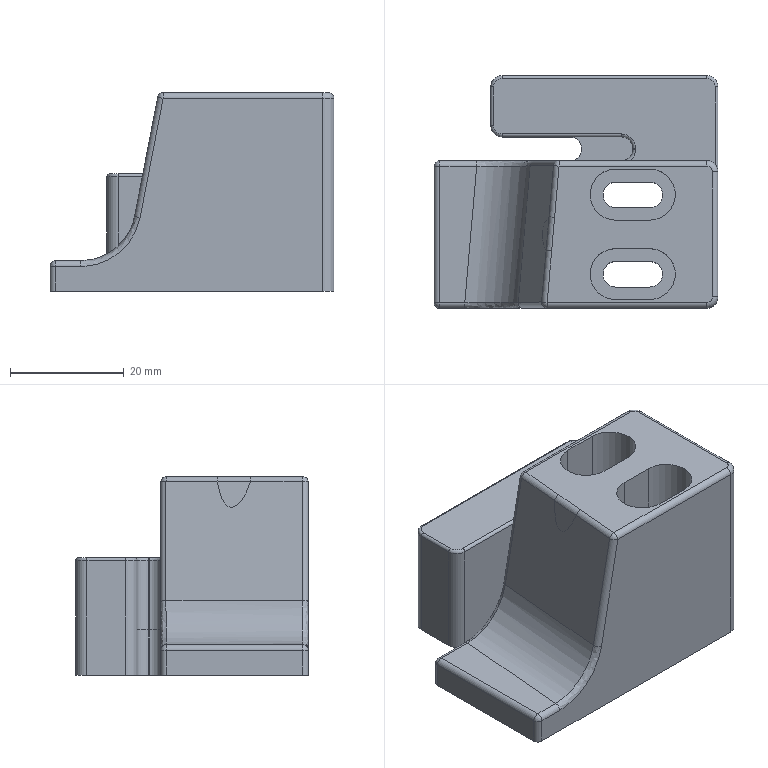NC program | NX | posted with a generic post | part box 50 x 41 x 35 mm
Lines 5590 to 6591 of 6591:
(CAVITY_MILL_COPY_COPY , TOOL : D4)
N11154 T04 M6
N11156 G17 G43 G0 G90 X-9.331 Y5.48 Z30. S9500 H4 M3
N11158 Z-14.738
N11160 G94 G1 X-9.129 Y5.481 F1000.
N11162 G3 X-8.265 Y5.984 R1.
N11164 G2 X-5.643 Y7.5 R3.011 F1400.
N11166 G1 X8.004
N11168 Y7.7
N11170 X8. Y7.704
N11172 X-9.144
N11174 G3 X-10.01 Y7.204 R1.
N11176 G1 X-10.184 Y6.904
N11178 G0 X-9.42 Y5.455 Z-15.177
N11180 G1 X-9.217 Y5.456 F1000.
N11182 G3 X-8.355 Y5.963 R1.
N11184 G2 X-5.728 Y7.5 R3.029 F1400.
N11186 G1 X8.
N11188 Y7.7
N11190 X-9.232
N11192 G3 X-10.098 Y7.2 R1.
N11194 G1 X-10.271 Y6.9
N11196 G0 X-9.505 Y5.452 Z-15.615
N11198 G1 X-9.303 Y5.454 F1000.
N11200 G3 X-8.441 Y5.962 R1.
N11202 G2 X-5.812 Y7.5 R3.03 F1400.
N11204 G1 X8.
N11206 Y7.7
N11208 X-9.317
N11210 G3 X-10.183 Y7.2 R1.
N11212 G1 X-10.356 Y6.9
N11214 G0 X-9.589 Y5.455 Z-16.054
N11216 G1 X-9.387 Y5.457 F1000.
N11218 G3 X-8.525 Y5.964 R1.
N11220 G2 X-5.863 Y7.5 R3.03 F1400.
N11222 G1 X8.
N11224 Y7.7
N11226 X-9.401
N11228 G3 X-10.267 Y7.2 R1.
N11230 G1 X-10.44 Y6.9
N11232 G0 X-9.671 Y5.476 Z-16.492
N11234 G1 X-9.469 Y5.477 F1000.
N11236 G3 X-8.606 Y5.981 R1.
N11238 G2 X-5.982 Y7.5 R3.011 F1400.
N11240 G1 X8.
N11242 Y7.7
N11244 X-9.486
N11246 G3 X-10.352 Y7.2 R1.
N11248 G1 X-10.525 Y6.9
N11250 G0 X-9.756 Y5.476 Z-16.931
N11252 G1 X-9.554 Y5.477 F1000.
N11254 G3 X-8.69 Y5.981 R1.
N11256 G2 X-6.067 Y7.5 R3.011 F1400.
N11258 G1 X8.
N11260 Y7.7
N11262 X-9.571
N11264 G3 X-10.437 Y7.2 R1.
N11266 G1 X-10.61 Y6.9
N11268 G0 X-9.843 Y5.457 Z-17.369
N11270 G1 X-9.641 Y5.459 F1000.
N11272 G3 X-8.778 Y5.966 R1.
N11274 G2 X-6.152 Y7.5 R3.028 F1400.
N11276 G1 X8.
N11278 Y7.7
N11280 X-9.655
N11282 G3 X-10.521 Y7.2 R1.
N11284 G1 X-10.695 Y6.9
N11286 G0 X-9.929 Y5.455 Z-17.808
N11288 G1 X-9.726 Y5.456 F1000.
N11290 G3 X-8.864 Y5.964 R1.
N11292 G2 X-6.202 Y7.5 R3.03 F1400.
N11294 G1 X8.
N11296 Y7.7
N11298 X-9.74
N11300 G3 X-10.606 Y7.2 R1.
N11302 G1 X-10.779 Y6.9
N11304 G0 X-10.013 Y5.455 Z-18.246
N11306 G1 X-9.81 Y5.456 F1000.
N11308 G3 X-8.948 Y5.964 R1.
N11310 G2 X-6.321 Y7.5 R3.03 F1400.
N11312 G1 X8.
N11314 Y7.7
N11316 X-9.825
N11318 G3 X-10.691 Y7.2 R1.
N11320 G1 X-10.864 Y6.9
N11322 G0 X-10.095 Y5.475 Z-18.685
N11324 G1 X-9.893 Y5.476 F1000.
N11326 G3 X-9.03 Y5.981 R1.
N11328 G2 X-6.406 Y7.5 R3.011 F1400.
N11330 G1 X8.
N11332 Y7.7
N11334 X-9.91
N11336 G3 X-10.776 Y7.2 R1.
N11338 G1 X-10.949 Y6.9
N11340 G0 X-10.184 Y5.449 Z-19.123
N11342 G1 X-9.98 Y5.451 F1000.
N11344 G3 X-9.119 Y5.959 R1.
N11346 G2 X-6.447 Y7.5 R3.035 F1400.
N11348 G1 X8.
N11350 Y7.7
N11352 X-9.994
N11354 G3 X-10.86 Y7.2 R1.
N11356 G1 X-11.034 Y6.9
N11358 G0 X-10.265 Y5.475 Z-19.562
N11360 G1 X-10.062 Y5.476 F1000.
N11362 G3 X-9.199 Y5.981 R1.
N11364 G2 X-6.575 Y7.5 R3.011 F1400.
N11366 G1 X8.
N11368 Y7.7
N11370 X-10.079
N11372 G3 X-10.945 Y7.2 R1.
N11374 G1 X-11.118 Y6.9
N11376 G0 X-10.351 Y5.455 Z-20.
N11378 G1 X-10.148 Y5.457 F1000.
N11380 G3 X-9.286 Y5.964 R1.
N11382 G2 X-6.659 Y7.5 R3.03 F1400.
N11384 G1 X8.
N11386 Y7.7
N11388 X-10.162
N11390 G3 X-11.029 Y7.2 R1.
N11392 G1 X-11.202 Y6.9
N11394 G0 X-10.437 Y5.453 Z-20.438
N11396 G1 X-10.234 Y5.455 F1000.
N11398 G3 X-9.372 Y5.962 R1.
N11400 G2 X-6.745 Y7.5 R3.031 F1400.
N11402 G1 X8.
N11404 Y7.7
N11406 X-10.248
N11408 G3 X-11.115 Y7.2 R1.
N11410 G1 X-11.288 Y6.9
N11412 G0 X-10.522 Y5.451 Z-20.875
N11414 G1 X-10.319 Y5.453 F1000.
N11416 G3 X-9.458 Y5.961 R1.
N11418 G2 X-6.794 Y7.5 R3.03 F1400.
N11420 G1 X8.
N11422 Y7.7
N11424 X-10.334
N11426 G3 X-11.2 Y7.2 R1.
N11428 G1 X-11.373 Y6.9
N11430 G0 X-10.606 Y5.465 Z-21.313
N11432 G1 X-10.404 Y5.466 F1000.
N11434 G3 X-9.542 Y5.973 R1.
N11436 G2 X-6.914 Y7.5 R3.011 F1400.
N11438 G1 X8.
N11440 Y7.7
N11442 X-10.421
N11444 G3 X-11.287 Y7.2 R1.
N11446 G1 X-11.46 Y6.9
N11448 G0 X-10.696 Y5.431 Z-21.75
N11450 G1 X-10.493 Y5.434 F1000.
N11452 G3 X-9.634 Y5.946 R1.
N11454 G2 X-6.998 Y7.5 R3.034 F1400.
N11456 G1 X8.
N11458 Y7.7
N11460 X-10.508
N11462 G3 X-11.374 Y7.2 R1.
N11464 G1 X-11.547 Y6.9
N11466 G0 X-10.788 Y5.443 Z-22.188
N11468 G1 X-10.586 Y5.446 F1000.
N11470 G3 X-9.727 Y5.958 R1.
N11472 G2 X-7.087 Y7.5 R3.013 F1400.
N11474 G1 X8.
N11476 Y7.7
N11478 X-10.604
N11480 G3 X-11.47 Y7.2 R1.
N11482 G1 X-11.643 Y6.9
N11484 G0 X-10.906 Y5.447 Z-22.625
N11486 G1 X-10.706 Y5.449 F1000.
N11488 G3 X-9.848 Y5.962 R1.
N11490 G2 X-8.516 Y7.198 R2.942 F1400.
N11492 G1 X-8.217 Y7.32
N11494 G2 X-7.189 Y7.5 R3.049
N11496 G1 X8.
N11498 Y7.7
N11500 X-10.726
N11502 G3 X-11.592 Y7.2 R1.
N11504 G1 X-11.765 Y6.9
N11506 G0 X-11.032 Y5.473 Z-23.063
N11508 G1 X-10.831 Y5.474 F1000.
N11510 G3 X-9.968 Y5.979 R1.
N11512 G2 X-8.017 Y7.418 R2.987 F1400.
N11514 X-7.311 Y7.5 R3.335
N11516 G1 X8.
N11518 Y7.7
N11520 X-10.847
N11522 G3 X-11.713 Y7.2 R1.
N11524 G1 X-11.887 Y6.9
N11526 G0 X-11.196 Y5.452 Z-23.5
N11528 G1 X-10.995 Y5.454 F1000.
N11530 G3 X-10.133 Y5.961 R1.
N11532 G2 X-8.477 Y7.32 R2.974 F1400.
N11534 X-7.454 Y7.5 R2.915
N11536 G1 X8.
N11538 Y7.7
N11540 X-11.008
N11542 G3 X-11.874 Y7.2 R1.
N11544 G1 X-12.047 Y6.9
N11546 G0 X-11.4 Y5.448 Z-23.938
N11548 G1 X-11.173 Y5.449 F1000.
N11550 G3 X-10.309 Y5.953 R1.
N11552 G2 X-7.618 Y7.5 R3.072 F1400.
N11554 G1 X8.
N11556 Y7.7
N11558 X-11.181
N11560 G3 X-12.047 Y7.2 R1.
N11562 G1 X-12.22 Y6.9
N11564 G0 X-11.591 Y5.532 Z-24.375
N11566 G1 X-11.431 Y5.519 F1000.
N11568 G3 X-10.527 Y5.947 R1.
N11570 G1 X-10.462 Y6.035 F1400.
N11572 G2 X-9.002 Y7.261 R2.886
N11574 G1 X-8.855 Y7.32
N11576 G2 X-7.805 Y7.5 R3.174
N11578 G1 X8.
N11580 Y7.7
N11582 X-11.392
N11584 G3 X-12.258 Y7.2 R1.
N11586 G1 X-12.431 Y6.9
N11588 G0 X-11.818 Y5.505 Z-24.813
N11590 G1 X-11.622 Y5.502 F1000.
N11592 G3 X-10.748 Y5.989 R1.
N11594 G2 X-9.805 Y6.948 R2.853 F1400.
N11596 G1 X-9.678 Y7.027
N11598 G2 X-8.02 Y7.5 R3.142
N11600 G1 X8.
N11602 Y7.7
N11604 X-11.618
N11606 G3 X-12.484 Y7.2 R1.
N11608 G1 X-12.657 Y6.9
N11610 G0 X-12.106 Y5.475 Z-25.25
N11612 G1 X-11.924 Y5.469 F1000.
N11614 G3 X-11.043 Y5.942 R1.
N11616 G1 X-10.949 Y6.084 F1400.
N11618 G2 X-8.254 Y7.5 R3.263
N11620 G1 X8.
N11622 Y7.7
N11624 X-11.896
N11626 G3 X-12.762 Y7.2 R1.
N11628 G1 X-12.935 Y6.9
N11630 G0 X-12.399 Y5.469 Z-25.688
N11632 G1 X-12.2 Y5.468 F1000.
N11634 G3 X-11.331 Y5.962 R1.
N11636 G2 X-10.441 Y6.907 R2.907 F1400.
N11638 X-8.518 Y7.5 R3.501
N11640 G1 X8.
N11642 Y7.7
N11644 X-12.198
N11646 G3 X-13.064 Y7.2 R1.
N11648 G1 X-13.234 Y6.906
N11650 G0 X-12.742 Y5.449 Z-26.125
N11652 G1 X-12.543 Y5.448 F1000.
N11654 G3 X-11.673 Y5.941 R1.
N11656 G2 X-10.343 Y7.131 R2.923 F1400.
N11658 G1 X-10.116 Y7.232
N11660 G2 X-8.855 Y7.5 R3.099
N11662 G1 X8.
N11664 Y7.7
N11666 X-12.532
N11668 G3 X-13.398 Y7.2 R1.
N11670 G1 X-13.553 Y6.932
N11672 G0 X-13.117 Y5.51 Z-26.563
N11674 G1 X-12.923 Y5.503 F1000.
N11676 G3 X-12.041 Y5.976 R1.
N11678 G2 X-11.64 Y6.48 R2.775 F1400.
N11680 X-9.168 Y7.5 R3.507
N11682 G1 X8.
N11684 Y7.7
N11686 X-12.898
N11688 G3 X-13.764 Y7.2 R1.
N11690 G1 X-13.889 Y6.983
N11692 G0 X-13.612 Y5.249 Z-27.
N11694 G1 X-13.423 Y5.255 F1000.
N11696 G3 X-12.574 Y5.784 R1.
N11698 G2 X-11.99 Y6.523 R2.671 F1400.
N11700 G1 X-11.922 Y6.584
N11702 G2 X-9.501 Y7.5 R3.521
N11704 G1 X8.
N11706 Y7.7
N11708 X-13.
N11710 G2 X-13.364 Y7.717 R4.
N11712 G3 X-14.272 Y7.297 R1.
N11714 G1 X-14.404 Y7.11
N11716 G0 X-14.044 Y5.519 Z-27.433
N11718 G1 X-13.85 Y5.511 F1000.
N11720 G3 X-12.964 Y5.974 R1.
N11722 G2 X-12.264 Y6.721 R2.766 F1400.
N11724 X-9.914 Y7.5 R4.031
N11726 G1 X-1.
N11728 Y7.614
N11730 Y7.7
N11732 X-13.
N11734 G2 X-13.704 Y7.762 R4.
N11736 G3 X-14.645 Y7.423 R1.
N11738 G1 X-14.793 Y7.247
N11740 G0 X-14.588 Y5.601 Z-27.867
N11742 G1 X-14.402 Y5.583 F1000.
N11744 G3 X-13.494 Y6.001 R1.
N11746 G2 X-13.249 Y6.298 R2.59 F1400.
N11748 X-10.335 Y7.5 R3.909
N11750 G1 X-1.
N11752 Y7.614
N11754 Y7.7
N11756 X-13.
N11758 G2 X-14.082 Y7.849 R4.
N11760 G3 X-15.051 Y7.602 R1.
N11762 G1 X-15.216 Y7.442
N11764 G0 X-15.192 Y5.797 Z-28.3
N11766 G1 X-15.008 Y5.768 F1000.
N11768 G3 X-14.074 Y6.126 R1.
N11770 G2 X-13.701 Y6.5 R2.589 F1400.
N11772 X-10.881 Y7.5 R4.428
N11774 G1 X-1.
N11776 Y7.614
N11778 Y7.7
N11780 X-13.
N11782 G2 X-14.5 Y7.992 R4.
N11784 G3 X-15.49 Y7.853 R1.
N11786 G1 X-15.671 Y7.712
N11788 G0 X-15.882 Y6.108 Z-28.733
N11790 G1 X-15.71 Y6.057 F1000.
N11792 G3 X-14.738 Y6.293 R1.
N11794 G1 X-14.686 Y6.34 F1400.
N11796 G2 X-11.471 Y7.5 R4.895
N11798 G1 X-1.
N11800 Y7.614
N11802 Y7.7
N11804 X-13.
N11806 G2 X-14.934 Y8.199 R4.
N11808 G3 X-15.934 Y8.18 R1.
N11810 G1 X-16.13 Y8.061
N11812 G0 X-16.711 Y6.539 Z-29.167
N11814 G1 X-16.521 Y6.444 F1000.
N11816 G3 X-15.523 Y6.505 R1.
N11818 G2 X-12.156 Y7.5 R5.991 F1400.
N11820 G1 X-1.
N11822 Y7.614
N11824 Y7.7
N11826 X-13.
N11828 G2 X-15.39 Y8.493 R4.
N11830 G3 X-16.383 Y8.609 R1.
N11832 G1 X-16.594 Y8.518
N11834 G0 X-17.348 Y7.461 Z-29.6
N11836 G1 X-17.132 Y7.248 F1000.
N11838 G3 X-16.164 Y6.996 R1.
N11840 G2 X-12.973 Y7.5 R14.382 F1400.
N11842 G1 X-1.
N11844 Y7.614
N11846 Y7.7
N11848 X-13.
N11850 G2 X-15.794 Y8.838 R4.
N11852 G3 X-16.763 Y9.085 R1.
N11854 G1 X-16.984 Y9.023
N11856 G0 X-17.842 Y8.135 Z-30.05
N11858 G1 X-17.648 Y7.827 F1000.
N11860 G3 X-16.764 Y7.36 R1.
N11862 X-14.121 Y7.5 R90.943 F1400.
N11864 G1 X-1.
N11866 Y7.614
N11868 Y7.7
N11870 X-13.
N11872 G2 X-16.087 Y9.156 R4.
N11874 G3 X-17.023 Y9.506 R1.
N11876 G1 X-17.25 Y9.468
N11878 G0 X-18.019 Y8.295 Z-30.5
N11880 G1 X-17.844 Y7.994 F1000.
N11882 G3 X-16.976 Y7.497 R1.
N11884 G1 X-16.048 Y7.5 F1400.
N11886 X-1.
N11888 Y7.614
N11890 Y7.7
N11892 X-13.
N11894 G2 X-16.186 Y9.281 R4.
N11896 G3 X-17.108 Y9.669 R1.
N11898 G1 X-17.335 Y9.64
N11900 G0 X-18.03 Y8.3 Z-30.95
N11902 G1 X-17.856 Y8. F1000.
N11904 G3 X-16.99 Y7.5 R1.
N11906 G1 X-1. F1400.
N11908 Y7.614
N11910 Y7.7
N11912 X-13.
N11914 G2 X-16.189 Y9.285 R4.
N11916 G3 X-17.11 Y9.674 R1.
N11918 G1 X-17.338 Y9.646
N11920 G0 X-18.03 Y8.3 Z-31.4
N11922 G1 X-17.856 Y8. F1000.
N11924 G3 X-16.99 Y7.5 R1.
N11926 G1 X-1. F1400.
N11928 Y7.614
N11930 Y7.7
N11932 X-13.
N11934 G2 X-16.189 Y9.285 R4.
N11936 G3 X-17.11 Y9.674 R1.
N11938 G1 X-17.338 Y9.646
N11940 G0 X-18.03 Y8.3 Z-31.85
N11942 G1 X-17.856 Y8. F1000.
N11944 G3 X-16.99 Y7.5 R1.
N11946 G1 X-1. F1400.
N11948 Y7.614
N11950 Y7.7
N11952 X-13.
N11954 G2 X-16.189 Y9.285 R4.
N11956 G3 X-17.11 Y9.674 R1.
N11958 G1 X-17.338 Y9.646
N11960 G0 X-18.03 Y8.3 Z-32.3
N11962 G1 X-17.856 Y8. F1000.
N11964 G3 X-16.99 Y7.5 R1.
N11966 G1 X-1. F1400.
N11968 Y7.614
N11970 Y7.7
N11972 X-13.
N11974 G2 X-16.189 Y9.285 R4.
N11976 G3 X-17.11 Y9.674 R1.
N11978 G1 X-17.338 Y9.646
N11980 G0 X-18.03 Y8.3 Z-32.75
N11982 G1 X-17.856 Y8. F1000.
N11984 G3 X-16.99 Y7.5 R1.
N11986 G1 X-1. F1400.
N11988 Y7.614
N11990 Y7.7
N11992 X-13.
N11994 G2 X-16.189 Y9.285 R4.
N11996 G3 X-17.11 Y9.674 R1.
N11998 G1 X-17.338 Y9.646
N12000 G0 X-18.03 Y8.3 Z-33.2
N12002 G1 X-17.856 Y8. F1000.
N12004 G3 X-16.99 Y7.5 R1.
N12006 G1 X-1. F1400.
N12008 Y7.614
N12010 Y7.7
N12012 X-13.
N12014 G2 X-16.189 Y9.285 R4.
N12016 G3 X-17.11 Y9.674 R1.
N12018 G1 X-17.338 Y9.646
N12020 G0 X-18.03 Y8.3 Z-33.65
N12022 G1 X-17.856 Y8. F1000.
N12024 G3 X-16.99 Y7.5 R1.
N12026 G1 X-1. F1400.
N12028 Y7.614
N12030 Y7.7
N12032 X-13.
N12034 G2 X-16.189 Y9.285 R4.
N12036 G3 X-17.11 Y9.674 R1.
N12038 G1 X-17.338 Y9.646
N12040 G0 X-18.03 Y8.3 Z-34.1
N12042 G1 X-17.856 Y8. F1000.
N12044 G3 X-16.99 Y7.5 R1.
N12046 G1 X-1. F1400.
N12048 Y7.614
N12050 Y7.7
N12052 X-13.
N12054 G2 X-16.189 Y9.285 R4.
N12056 G3 X-17.11 Y9.674 R1.
N12058 G1 X-17.338 Y9.646
N12060 G0 X-18.03 Y8.3 Z-34.55
N12062 G1 X-17.856 Y8. F1000.
N12064 G3 X-16.99 Y7.5 R1.
N12066 G1 X-1.001 F1400.
N12068 X-1. Y7.614
N12070 Y7.7
N12072 X-13.
N12074 G2 X-16.189 Y9.285 R4.
N12076 G3 X-17.11 Y9.674 R1.
N12078 G1 X-17.338 Y9.646
N12080 G0 X-18.03 Y8.3 Z-35.
N12082 G1 X-17.856 Y8. F1000.
N12084 G3 X-16.99 Y7.5 R1.
N12086 G1 X-1.001 F1400.
N12088 X-1. Y7.614
N12090 Y7.7
N12092 X-13.
N12094 G2 X-16.189 Y9.285 R4.
N12096 G3 X-17.11 Y9.674 R1.
N12098 G1 X-17.338 Y9.646
N12100 G0 Z30.
N12102 M5
(ZLEVEL_PROFILE_COPY_COPY_1_COPY_1 , TOOL : D6R0.5)
N12104 T08 M6
N12106 G54
N12108 G17 G0 G90 X-12.191 Y-24.7 S9500 M3
N12110 G43 Z30. H8
N12112 Z-28.112
N12114 G94 G1 Z-29.612 F1000.
N12116 X-12.711 Y-23.8
N12118 G3 X-13.23 Y-23.5 R0.6
N12120 G1 X-14.155 F3000.
N12122 G2 X-17.003 Y-23.081 R11.427
N12124 X-18.899 Y-22.487 R25.07
N12126 G1 X-19.061 Y-22.422
N12128 X-19.684 Y-22.208
N12130 X-19.79 Y-22.19
N12132 X-24.
N12134 G2 X-26.69 Y-19.5 R2.69
N12136 G1 Y4.5
N12138 G2 X-24. Y7.19 R2.69
N12140 G1 X-17.663
N12142 X-16.058 Y7.744
N12144 X-16.08 Y7.761 Z-29.618
N12146 X-16.079 Z-29.63
N12148 X-16.106 Y7.744
N12150 X-17.491 Y7.315
N12152 X-17.587 Y7.3
N12154 X-24.
N12156 G3 X-26.8 Y4.5 R2.8
N12158 G1 Y-19.5
N12160 G3 X-24. Y-22.3 R2.8
N12162 G1 X-19.638
N12164 Y-22.287
N12166 X-19.061 Y-22.47
N12168 X-19.018 Y-22.487
N12170 G3 X-17.003 Y-23.095 R29.857
N12172 X-14.178 Y-23.5 R11.584
N12174 G1 Z-29.655
N12176 G2 X-16.317 Y-23.267 R10.682
N12178 G1 X-16.66 Y-23.197
N12180 X-16.768 Y-23.176
N12182 X-17.003 Y-23.113
N12184 X-17.346 Y-23.028
N12186 X-18.718 Y-22.625
N12188 X-19.589 Y-22.403
N12190 X-24.
N12192 G2 X-26.903 Y-19.5 R2.903
N12194 G1 Y4.5
N12196 G2 X-24. Y7.403 R2.903
N12198 G1 X-17.496
N12200 X-17.346 Y7.418
N12202 X-16.317 Y7.716
N12204 X-16.107 Y7.782
N12206 X-16.109
N12208 X-16.145 Y7.813 Z-29.666
N12210 Z-29.686
N12212 G2 X-17.496 Y7.502 R5.293
N12214 G1 X-24.
N12216 G3 X-27.002 Y4.5 R3.002
N12218 G1 Y-19.5
N12220 G3 X-24. Y-22.502 R3.002
N12222 G1 X-19.589
N12224 G2 X-19.024 Y-22.595 R2.82
N12226 G1 X-17.346 Y-23.053
N12228 X-17.003 Y-23.136
N12230 G3 X-14.178 Y-23.5 R12.037
N12232 G1 Z-29.724
N12234 G2 X-16.437 Y-23.279 R11.409
N12236 X-18.718 Y-22.733 R31.316
N12238 G3 X-19.589 Y-22.597 R3.383
N12240 G1 X-24.
N12242 G2 X-27.097 Y-19.5 R3.097
N12244 G1 Y4.5
N12246 G2 X-24. Y7.597 R3.097
N12248 G1 X-17.496
N12250 G3 X-16.19 Y7.85 R4.229
N12252 G1 X-16.192 Y7.849
N12254 X-16.239 Y7.891 Z-29.738
N12256 Z-29.767
N12258 G2 X-17.496 Y7.689 R4.485
N12260 G1 X-24.
N12262 G3 X-27.189 Y4.5 R3.189
N12264 G1 Y-19.5
N12266 G3 X-24. Y-22.689 R3.189
N12268 G1 X-19.489
N12270 G2 X-18.81 Y-22.773 R2.766
N12272 G3 X-16.501 Y-23.289 R41.448
N12274 X-14.178 Y-23.5 R11.622
N12276 G1 Z-29.817
N12278 G2 X-16.532 Y-23.308 R12.557
N12280 X-18.375 Y-22.931 R36.058
N12282 G3 X-19.589 Y-22.777 R5.48
N12284 G1 X-24.
N12286 G2 X-27.277 Y-19.5 R3.277
N12288 G1 Y4.5
N12290 G2 X-24. Y7.777 R3.277
N12292 G1 X-17.496
N12294 X-17.346 Y7.773
N12296 X-16.357 Y7.914
N12298 X-16.292 Y7.937
N12300 X-16.294 Y7.936
N12302 X-16.348 Y7.987 Z-29.835
N12304 Z-29.872
N12306 G2 X-17.496 Y7.861 R5.248
N12308 G1 X-24.
N12310 G3 X-27.361 Y4.5 R3.361
N12312 G1 Y-19.5
N12314 G3 X-24. Y-22.861 R3.361
N12316 G1 X-19.589
N12318 G2 X-18.718 Y-22.932 R4.481
N12320 G1 X-17.003 Y-23.257
N12322 G3 X-14.178 Y-23.5 R14.483
N12324 G1 Z-29.932
N12326 G2 X-17.346 Y-23.231 R15.955
N12328 G3 X-19.061 Y-22.963 R23.316
N12330 G1 X-19.589 Y-22.942
N12332 X-24.
N12334 G2 X-27.442 Y-19.5 R3.442
N12336 G1 Y4.5
N12338 G2 X-24. Y7.942 R3.442
N12340 G1 X-17.496
N12342 G3 X-16.405 Y8.039 R5.61
N12344 X-16.99 Y8.173 R0.6
N12346 G1 X-18.648 Y9.142
N12348 Z-28.432
N12350 G0 Z30.
N12352 X-16.483 Y8.113
N12354 Z-28.432
N12356 G1 Z-29.998 F1000.
N12358 X-16.467 Y8.085 F3000.
N12360 X-16.487 Y8.08
N12362 G2 X-17.496 Y8.018 R7.797
N12364 G1 X-24.
N12366 G3 X-27.518 Y4.5 R3.518
N12368 G1 Y-19.5
N12370 G3 X-24. Y-23.018 R3.518
N12372 G1 X-19.589
N12374 G2 X-18.375 Y-23.109 R8.254
N12376 G1 X-17.003 Y-23.321
N12378 G3 X-14.178 Y-23.5 R16.73
N12380 G1 Z-30.069
N12382 G2 X-15.974 Y-23.458 R21.56
N12384 X-18.032 Y-23.21 R36.789
N12386 G3 X-19.589 Y-23.089 R11.421
N12388 G1 X-24.
N12390 G2 X-27.589 Y-19.5 R3.589
N12392 G1 Y4.5
N12394 G2 X-24. Y8.089 R3.589
N12396 G1 X-17.496
N12398 X-17.346 Y8.082
N12400 X-16.66 Y8.123
N12402 X-16.51 Y8.139
N12404 X-16.567 Y8.197 Z-30.144
N12406 X-17.346 Y8.15
N12408 X-17.496 Y8.156
N12410 X-24.
N12412 G3 X-27.656 Y4.5 R3.656
N12414 G1 Y-19.5
N12416 G3 X-24. Y-23.156 R3.656
N12418 G1 X-19.589
N12420 G2 X-17.621 Y-23.307 R15.254
N12422 G3 X-15.136 Y-23.496 R19.128
N12424 X-14.178 Y-23.5 R69.842
N12426 G1 X-14.259 Z-30.223
N12428 X-15.631 Y-23.497
N12430 G2 X-17.689 Y-23.341 R27.956
N12432 G3 X-19.589 Y-23.217 R16.569
N12434 G1 X-24.
N12436 G2 X-27.717 Y-19.5 R3.717
N12438 G1 Y4.5
N12440 G2 X-24. Y8.217 R3.717
N12442 G1 X-17.248
N12444 G3 X-16.62 Y8.251 R5.816
N12446 G1 X-16.662 Y8.296 Z-30.307
N12448 X-17.346 Y8.273
N12450 X-17.496
N12452 X-24.
N12454 G3 X-27.773 Y4.5 R3.773
N12456 G1 Y-19.5
N12458 G3 X-24. Y-23.273 R3.773
N12460 G1 X-19.496
N12462 G2 X-18.438 Y-23.315 R13.366
N12464 G1 X-16.66 Y-23.456
N12466 X-16.317 Y-23.479
N12468 G3 X-14.602 Y-23.5 R45.476
N12470 G1 Z-30.393
N12472 X-14.822 Y-23.498
N12474 X-15.554 Y-23.497
N12476 G2 X-17.834 Y-23.399 R27.121
N12478 G3 X-19.589 Y-23.323 R20.919
N12480 G1 X-24.
N12482 G2 X-27.823 Y-19.5 R3.823
N12484 G1 Y4.5
N12486 G2 X-24. Y8.323 R3.823
N12488 G1 X-17.496
N12490 X-17.346 Y8.322
N12492 X-16.745 Y8.337
N12494 X-16.703 Y8.34
N12496 X-16.74 Y8.382 Z-30.483
N12498 X-17.346 Y8.364
N12500 X-17.496 Y8.367
N12502 X-24.
N12504 G3 X-27.867 Y4.5 R3.867
N12506 G1 Y-19.5
N12508 G3 X-24. Y-23.367 R3.867
N12510 G1 X-19.324
N12512 G2 X-18.63 Y-23.385 R13.615
N12514 G1 X-16.66 Y-23.486
N12516 X-16.317 Y-23.497
N12518 X-14.822 Y-23.498
N12520 X-14.721 Y-23.5
N12522 X-14.821 Z-30.53
N12524 X-14.92 Y-23.498 Z-30.576
N12526 G2 X-18.164 Y-23.44 R51.79
N12528 G3 X-19.579 Y-23.405 R28.747
N12530 G1 X-24.
N12532 G2 X-27.905 Y-19.5 R3.905
N12534 G1 Y4.5
N12536 G2 X-24. Y8.405 R3.905
N12538 G1 X-17.496
N12540 X-16.803 Y8.409
N12542 X-16.769 Y8.415
N12544 X-16.792 Y8.441 Z-30.671
N12546 X-16.93 Y8.436
N12548 X-17.496 Y8.437
N12550 X-24.
N12552 G3 X-27.937 Y4.5 R3.937
N12554 G1 Y-19.5
N12556 G3 X-24. Y-23.437 R3.937
N12558 G1 X-19.387
N12560 G2 X-17.765 Y-23.474 R35.705
N12562 G1 X-17.689 Y-23.478
N12564 G3 X-15.133 Y-23.498 R67.033
N12566 G1 X-15.299 Y-23.5 Z-30.703
N12568 X-15.465 Z-30.735
N12570 X-15.631 Z-30.768
N12572 X-17.346 Y-23.497
N12574 X-18.788 Y-23.463
N12576 X-18.834
N12578 X-24.
N12580 G2 X-27.963 Y-19.5 R3.963
N12582 G1 Y4.5
N12584 G2 X-24. Y8.463 R3.963
N12586 G1 X-17.496
N12588 X-16.855 Y8.467
N12590 X-16.815 Y8.468
N12592 X-16.826 Y8.481 Z-30.851
N12594 X-17.496 Y8.479
N12596 X-24.
N12598 G3 X-27.979 Y4.5 R3.979
N12600 G1 Y-19.5
N12602 G3 X-24. Y-23.479 R3.979
N12604 G1 X-19.589
N12606 X-19.404 Y-23.471
N12608 X-18.375 Y-23.482
N12610 X-17.689 Y-23.497
N12612 X-15.631 Y-23.5
N12614 X-15.803 Z-30.892
N12616 X-15.974 Z-30.934
N12618 X-18.718 Y-23.49
N12620 X-19.292 Y-23.483
N12622 G3 X-19.589 Y-23.491 R4.208
N12624 G1 X-24.
N12626 G2 X-27.991 Y-19.5 R3.991
N12628 G1 Y4.5
N12630 G2 X-24. Y8.491 R3.991
N12632 G1 X-17.496
N12634 X-16.835 Y8.492
N12636 X-16.84 Y8.497 Z-31.017
N12638 X-16.918
N12640 X-17.496 Y8.498
N12642 X-24.
N12644 G3 X-27.998 Y4.5 R3.998
N12646 G1 Y-19.5
N12648 X-27.985 Y-19.814
N12650 G3 X-24. Y-23.498 R3.998
N12652 G1 X-19.589
N12654 X-16.317 Y-23.5
N12656 Z-31.1
N12658 X-19.061
N12660 X-19.404 Y-23.497
N12662 X-24.01 Y-23.498
N12664 X-24.411 Y-23.491
N12666 G2 X-25.751 Y-23.094 R4.668
N12668 X-27.952 Y-20.1 R3.993
N12670 G1 X-27.985 Y-19.814
N12672 X-27.998 Y-19.5
N12674 Y4.393
N12676 X-27.991 Y4.737
N12678 G2 X-26.993 Y7.15 R3.983
N12680 X-24. Y8.5 R3.996
N12682 G1 X-16.841 Y8.499
N12684 G3 X-17.404 Y8.706 R0.6
N12686 G1 X-18.868 Y9.699
N12688 Z-29.6
N12690 G0 Z30.
N12692 M5
(ZLEVEL_PROFILE_COPY_COPY_1_COPY_1_COPY , TOOL : D4R0.5)
N12694 T05 M6
N12696 G54
N12698 G17 G0 G90 X8.823 Y7.5 S9500 M3
N12700 G43 Z30. H5
N12702 Z-12.8
N12704 G94 G1 Z-14.316 F1000.
N12706 Y7.7 F3000.
N12708 G3 X8. Y8.523 R0.823
N12710 G1 X-13.
N12712 G2 X-16.177 Y11.7 R3.177
N12714 G1 Y18.5
N12716 G2 X-13. Y21.677 R3.177
N12718 G1 X23.
N12720 G2 X26.177 Y18.5 R3.177
N12722 G1 Y5.931
N12724 X26.236 Y5.859 Z-14.328
N12726 X26.282 Y5.787 Z-14.341
N12728 Y18.5
N12730 G3 X23. Y21.782 R3.282
N12732 G1 X-13.
N12734 G3 X-16.282 Y18.5 R3.282
N12736 G1 Y11.7
N12738 G3 X-13. Y8.418 R3.282
N12740 G1 X8.
N12742 G2 X8.718 Y7.7 R0.718
N12744 G1 Y7.5
N12746 X8.62 Z-14.375
N12748 Y7.7
N12750 G3 X8. Y8.32 R0.62
N12752 G1 X-13.
N12754 G2 X-16.38 Y11.7 R3.38
N12756 G1 Y18.5
N12758 G2 X-13. Y21.88 R3.38
N12760 G1 X23.
N12762 G2 X26.38 Y18.5 R3.38
N12764 G1 Y5.639
N12766 X26.43 Y5.562 Z-14.397
N12768 X26.473 Y5.485 Z-14.419
N12770 Y18.5
N12772 G3 X23. Y21.973 R3.473
N12774 G1 X-13.
N12776 G3 X-16.473 Y18.5 R3.473
N12778 G1 Y11.7
N12780 G3 X-13. Y8.227 R3.473
N12782 G1 X8.
N12784 G2 X8.527 Y7.7 R0.527
N12786 G1 Y7.5
N12788 X8.44 Z-14.471
N12790 Y7.7
N12792 G3 X8. Y8.14 R0.44
N12794 G1 X-13.
N12796 G2 X-16.56 Y11.7 R3.56
N12798 G1 Y18.5
N12800 G2 X-13. Y22.06 R3.56
N12802 G1 X23.
N12804 G2 X26.56 Y18.5 R3.56
N12806 G1 Y5.324
N12808 X26.602 Y5.241 Z-14.502
N12810 X26.64 Y5.157 Z-14.532
N12812 Y18.5
N12814 G3 X23. Y22.14 R3.64
N12816 G1 X-13.
N12818 G3 X-16.64 Y18.5 R3.64
N12820 G1 Y11.7
N12822 G3 X-13. Y8.06 R3.64
N12824 G1 X8.
N12826 G2 X8.36 Y7.7 R0.36
N12828 G1 Y7.5
N12830 X8.286 Z-14.6
N12832 Y7.7
N12834 G3 X8. Y7.986 R0.286
N12836 G1 X-13.
N12838 G2 X-16.714 Y11.7 R3.714
N12840 G1 Y18.5
N12842 G2 X-13. Y22.214 R3.714
N12844 G1 X23.
N12846 G2 X26.714 Y18.5 R3.714
N12848 G1 Y4.984
N12850 X26.749 Y4.895 Z-14.638
N12852 X26.781 Y4.805 Z-14.676
N12854 Y18.5
N12856 G3 X23. Y22.281 R3.781
N12858 G1 X-13.
N12860 G3 X-16.781 Y18.5 R3.781
N12862 G1 Y11.7
N12864 G3 X-13. Y7.919 R3.781
N12866 G1 X8.
N12868 G2 X8.219 Y7.7 R0.219
N12870 G1 Y7.5
N12872 X8.16 Z-14.757
N12874 Y7.7
N12876 G3 X8. Y7.86 R0.16
N12878 G1 X-13.
N12880 G2 X-16.84 Y11.7 R3.84
N12882 G1 Y18.5
N12884 G2 X-13. Y22.34 R3.84
N12886 G1 X23.
N12888 G2 X26.84 Y18.5 R3.84
N12890 G1 Y4.621
N12892 X26.866 Y4.526 Z-14.801
N12894 X26.89 Y4.432 Z-14.844
N12896 Y18.5
N12898 G3 X23. Y22.39 R3.89
N12900 G1 X-13.
N12902 G3 X-16.89 Y18.5 R3.89
N12904 G1 Y11.7
N12906 G3 X-13. Y7.81 R3.89
N12908 G1 X8.
N12910 X8.06 Y7.804
N12912 X8.104 Y7.76
N12914 X8.11 Y7.7
N12916 Y7.5
N12918 X8.069 Z-14.935
N12920 Y7.7
N12922 X8.068 Y7.739
N12924 X8.039 Y7.768
N12926 X8. Y7.769
N12928 X-13.
N12930 G2 X-16.931 Y11.7 R3.931
N12932 G1 Y18.5
N12934 G2 X-13. Y22.431 R3.931
N12936 G1 X23.
N12938 G2 X26.931 Y18.5 R3.931
N12940 G1 Y4.239
N12942 X26.948 Y4.145 Z-14.981
N12944 X26.962 Y4.051 Z-15.026
N12946 Y18.5
N12948 G3 X23. Y22.462 R3.962
N12950 G1 X-13.
N12952 G3 X-16.962 Y18.5 R3.962
N12954 G1 Y11.7
N12956 G3 X-13. Y7.738 R3.962
N12958 G1 X8.
N12960 X8.024 Y7.742
N12962 X8.042 Y7.724
N12964 X8.038 Y7.7
N12966 Y7.5
N12968 X7.534
N12970 X7.47
N12972 X7.417 Y7.499
N12974 Z-15.118
N12976 X7.461 Y7.5
N12978 X7.98
N12980 X8.017
N12982 Y7.7
N12984 X8.018 Y7.718
N12986 X8. Y7.717
N12988 X-13.
N12990 G2 X-16.983 Y11.7 R3.983
N12992 G1 Y18.5
N12994 G2 X-13. Y22.483 R3.983
N12996 G1 X23.
N12998 G2 X26.983 Y18.5 R3.983
N13000 G1 Y3.866
N13002 X26.993 Y3.728 Z-15.163
N13004 X26.996 Y3.591 Z-15.209
N13006 Y18.5
N13008 G3 X23. Y22.496 R3.996
N13010 G1 X-13.
N13012 G3 X-16.996 Y18.5 R3.996
N13014 G1 Y11.7
N13016 G3 X-13. Y7.704 R3.996
N13018 G1 X8.
N13020 X8.004
N13022 Y7.7
N13024 Y7.5
N13026 X7.461
N13028 X7.417 Y7.499
N13030 X7.4 Y7.5 Z-15.3
N13032 X7.987 Y7.501
N13034 X7.999 Y7.504
N13036 X8. Y7.671
N13038 X7.999 Y7.699
N13040 X-12.937 Y7.702
N13042 G2 X-16.998 Y11.69 R4.
N13044 G1 Y18.449
N13046 G2 X-13. Y22.5 R4.001
N13048 G1 X23.
N13050 G2 X27. Y18.5 R4.002
N13052 G1 Y1.881
N13054 G3 X27.2 Y1.535 R0.4
N13056 G1 X27.8 Y1.188
N13058 Z-13.8
N13060 G0 Z30.
N13062 M5
(ZLEVEL_PROFILE_1_COPY_1_COPY_COPY , TOOL : D4A45)
N13064 T02 M6
N13066 G54
N13068 G17 G0 G90 X6.246 Y-17.136 S9500 M3
N13070 G43 Z30. H2
N13072 Z0.
N13074 G94 G1 Z-1. F1000.
N13076 X6.654 Y-17.841
N13078 G3 X7. Y-18.041 R0.4
N13080 G1 X13.
N13082 G3 X16.541 Y-14.5 R3.541
N13084 X13. Y-10.959 R3.541
N13086 G1 X7.
N13088 G3 X3.459 Y-14.5 R3.541
N13090 X7. Y-18.041 R3.541
N13092 X7.346 Y-17.841 R0.4
N13094 G1 X7.693 Y-17.241
N13096 Z0.
N13098 G0 Z30.
N13100 X6.246 Y-3.136
N13102 Z0.
N13104 G1 Z-1.
N13106 X6.654 Y-3.841
N13108 G3 X7. Y-4.041 R0.4
N13110 G1 X13.
N13112 G3 X16.541 Y-0.5 R3.541
N13114 X13. Y3.041 R3.541
N13116 G1 X7.
N13118 G3 X3.459 Y-0.5 R3.541
N13120 X7. Y-4.041 R3.541
N13122 X7.346 Y-3.841 R0.4
N13124 G1 X7.693 Y-3.241
N13126 Z0.
N13128 G0 Z30.
N13130 M5
N13132 M2